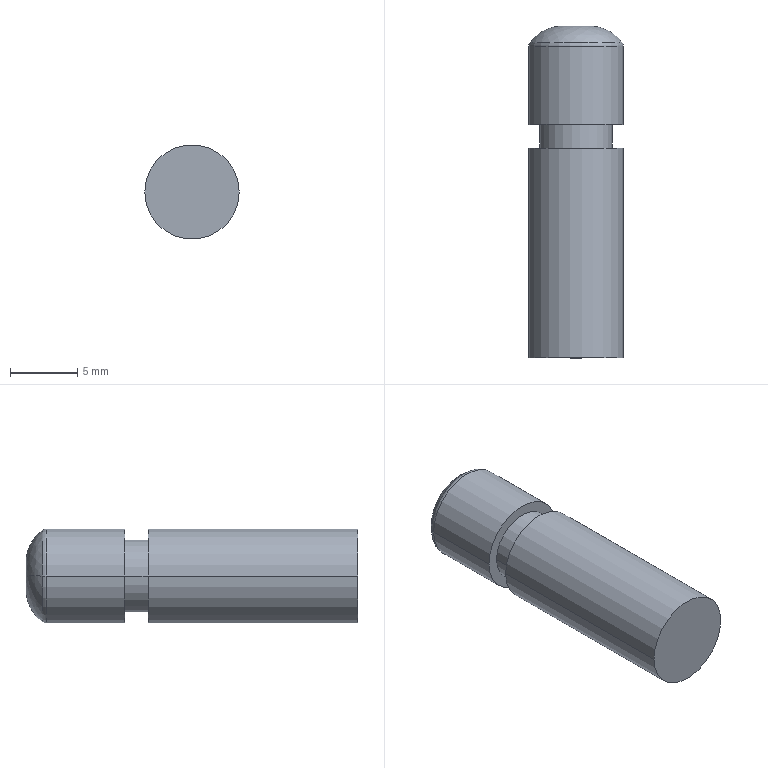Part | STEP file | 2023_07_21_12_39_19_0133 | 1 solid | 14 faces | box 7 x 24.6 x 7 mm | volume 901.225 mm3 | cylinder 6 | plane 4 | spline 2 | torus 2 | commonest cylinder face diameters 7 x4 5.4 x2
STEP:
#1=CARTESIAN_POINT('',(16.5,75.7,12.5));
#2=VERTEX_POINT('',#1);
#3=CARTESIAN_POINT('',(14.5,75.7,12.5));
#4=VERTEX_POINT('',#3);
#5=CARTESIAN_POINT('',(15.5,75.7,12.5));
#6=DIRECTION('',(0.,-1.,0.));
#7=DIRECTION('',(-1.,0.,0.));
#8=AXIS2_PLACEMENT_3D('',#5,#6,#7);
#9=CIRCLE('',#8,1.);
#10=EDGE_CURVE('',#2,#4,#9,.T.);
#11=ORIENTED_EDGE('',*,*,#10,.T.);
#12=CARTESIAN_POINT('',(12.1,74.5,12.5));
#13=VERTEX_POINT('',#12);
#14=CARTESIAN_POINT('',(14.5,75.7,12.5));
#15=CARTESIAN_POINT('',(13.,75.7,12.5));
#16=CARTESIAN_POINT('',(12.1,74.5,12.5));
#17=(BOUNDED_CURVE()B_SPLINE_CURVE(2,(#14,#15,#16),.UNSPECIFIED.,.F.,.F.)B_SPLINE_CURVE_WITH_KNOTS((3,3),(-1.571,-0.6435),.UNSPECIFIED.)CURVE()GEOMETRIC_REPRESENTATION_ITEM()RATIONAL_B_SPLINE_CURVE((1.,0.8944,1.))REPRESENTATION_ITEM(''));
#18=EDGE_CURVE('',#4,#13,#17,.T.);
#19=ORIENTED_EDGE('',*,*,#18,.T.);
#20=CARTESIAN_POINT('',(18.9,74.5,12.5));
#21=VERTEX_POINT('',#20);
#22=CARTESIAN_POINT('',(15.5,74.5,12.5));
#23=DIRECTION('',(0.,-1.,0.));
#24=DIRECTION('',(-1.,0.,0.));
#25=AXIS2_PLACEMENT_3D('',#22,#23,#24);
#26=CIRCLE('',#25,3.4);
#27=EDGE_CURVE('',#21,#13,#26,.T.);
#28=ORIENTED_EDGE('',*,*,#27,.F.);
#29=CARTESIAN_POINT('',(16.5,75.7,12.5));
#30=CARTESIAN_POINT('',(18.,75.7,12.5));
#31=CARTESIAN_POINT('',(18.9,74.5,12.5));
#32=(BOUNDED_CURVE()B_SPLINE_CURVE(2,(#29,#30,#31),.UNSPECIFIED.,.F.,.F.)B_SPLINE_CURVE_WITH_KNOTS((3,3),(-1.571,-0.6435),.UNSPECIFIED.)CURVE()GEOMETRIC_REPRESENTATION_ITEM()RATIONAL_B_SPLINE_CURVE((1.,0.8944,1.))REPRESENTATION_ITEM(''));
#33=EDGE_CURVE('',#2,#21,#32,.T.);
#34=ORIENTED_EDGE('',*,*,#33,.F.);
#35=EDGE_LOOP('',(#11,#19,#28,#34));
#36=FACE_OUTER_BOUND('',#35,.T.);
#37=CARTESIAN_POINT('',(16.5,75.7,12.5));
#38=CARTESIAN_POINT('',(16.5,75.7,13.5));
#39=CARTESIAN_POINT('',(15.5,75.7,13.5));
#40=CARTESIAN_POINT('',(14.5,75.7,13.5));
#41=CARTESIAN_POINT('',(14.5,75.7,12.5));
#42=CARTESIAN_POINT('',(14.5,75.7,11.5));
#43=CARTESIAN_POINT('',(15.5,75.7,11.5));
#44=CARTESIAN_POINT('',(16.5,75.7,11.5));
#45=CARTESIAN_POINT('',(16.5,75.7,12.5));
#46=CARTESIAN_POINT('',(18.,75.7,12.5));
#47=CARTESIAN_POINT('',(18.,75.7,15.));
#48=CARTESIAN_POINT('',(15.5,75.7,15.));
#49=CARTESIAN_POINT('',(13.,75.7,15.));
#50=CARTESIAN_POINT('',(13.,75.7,12.5));
#51=CARTESIAN_POINT('',(13.,75.7,10.));
#52=CARTESIAN_POINT('',(15.5,75.7,10.));
#53=CARTESIAN_POINT('',(18.,75.7,10.));
#54=CARTESIAN_POINT('',(18.,75.7,12.5));
#55=CARTESIAN_POINT('',(18.9,74.5,12.5));
#56=CARTESIAN_POINT('',(18.9,74.5,15.9));
#57=CARTESIAN_POINT('',(15.5,74.5,15.9));
#58=CARTESIAN_POINT('',(12.1,74.5,15.9));
#59=CARTESIAN_POINT('',(12.1,74.5,12.5));
#60=CARTESIAN_POINT('',(12.1,74.5,9.1));
#61=CARTESIAN_POINT('',(15.5,74.5,9.1));
#62=CARTESIAN_POINT('',(18.9,74.5,9.1));
#63=CARTESIAN_POINT('',(18.9,74.5,12.5));
#64=(BOUNDED_SURFACE()B_SPLINE_SURFACE(2,2,((#37,#38,#39,#40,#41,#42,#43,#44,#45),(#46,#47,#48,#49,#50,#51,#52,#53,#54),(#55,#56,#57,#58,#59,#60,#61,#62,#63)),.UNSPECIFIED.,.F.,.T.,.F.)B_SPLINE_SURFACE_WITH_KNOTS((3,3),(3,2,2,2,3),(-1.571,-0.6435),(-3.142,-1.571,0.,1.571,3.142),.UNSPECIFIED.)GEOMETRIC_REPRESENTATION_ITEM()RATIONAL_B_SPLINE_SURFACE(((1.,0.7071,1.,0.7071,1.,0.7071,1.,0.7071,1.),(0.8944,0.6325,0.8944,0.6325,0.8944,0.6325,0.8944,0.6325,0.8944),(1.,0.7071,1.,0.7071,1.,0.7071,1.,0.7071,1.)))REPRESENTATION_ITEM('')SURFACE());
#65=ADVANCED_FACE('',(#36),#64,.F.);
#66=CARTESIAN_POINT('',(19.,51.1,12.5));
#67=VERTEX_POINT('',#66);
#68=CARTESIAN_POINT('',(12.,51.1,12.5));
#69=VERTEX_POINT('',#68);
#70=CARTESIAN_POINT('',(15.5,51.1,12.5));
#71=DIRECTION('',(0.,-1.,0.));
#72=DIRECTION('',(-1.,0.,0.));
#73=AXIS2_PLACEMENT_3D('',#70,#71,#72);
#74=CIRCLE('',#73,3.5);
#75=EDGE_CURVE('',#67,#69,#74,.T.);
#76=ORIENTED_EDGE('',*,*,#75,.F.);
#77=CARTESIAN_POINT('',(19.,66.65,12.5));
#78=VERTEX_POINT('',#77);
#79=CARTESIAN_POINT('',(19.,58.875,12.5));
#80=DIRECTION('',(0.,1.,0.));
#81=VECTOR('',#80,1000.);
#82=LINE('',#79,#81);
#83=EDGE_CURVE('',#67,#78,#82,.T.);
#84=ORIENTED_EDGE('',*,*,#83,.T.);
#85=CARTESIAN_POINT('',(12.,66.65,12.5));
#86=VERTEX_POINT('',#85);
#87=CARTESIAN_POINT('',(15.5,66.65,12.5));
#88=DIRECTION('',(0.,-1.,0.));
#89=DIRECTION('',(-1.,0.,0.));
#90=AXIS2_PLACEMENT_3D('',#87,#88,#89);
#91=CIRCLE('',#90,3.5);
#92=EDGE_CURVE('',#78,#86,#91,.T.);
#93=ORIENTED_EDGE('',*,*,#92,.T.);
#94=CARTESIAN_POINT('',(12.,58.875,12.5));
#95=DIRECTION('',(0.,1.,0.));
#96=VECTOR('',#95,1000.);
#97=LINE('',#94,#96);
#98=EDGE_CURVE('',#69,#86,#97,.T.);
#99=ORIENTED_EDGE('',*,*,#98,.F.);
#100=EDGE_LOOP('',(#76,#84,#93,#99));
#101=FACE_OUTER_BOUND('',#100,.T.);
#102=CARTESIAN_POINT('',(15.5,58.875,12.5));
#103=DIRECTION('',(0.,1.,0.));
#104=DIRECTION('',(-1.,0.,0.));
#105=AXIS2_PLACEMENT_3D('',#102,#103,#104);
#106=CYLINDRICAL_SURFACE('',#105,3.5);
#107=ADVANCED_FACE('',(#101),#106,.T.);
#108=CARTESIAN_POINT('',(18.2,66.65,12.5));
#109=VERTEX_POINT('',#108);
#110=CARTESIAN_POINT('',(12.8,66.65,12.5));
#111=VERTEX_POINT('',#110);
#112=CARTESIAN_POINT('',(15.5,66.65,12.5));
#113=DIRECTION('',(0.,-1.,0.));
#114=DIRECTION('',(-1.,0.,0.));
#115=AXIS2_PLACEMENT_3D('',#112,#113,#114);
#116=CIRCLE('',#115,2.7);
#117=EDGE_CURVE('',#109,#111,#116,.T.);
#118=ORIENTED_EDGE('',*,*,#117,.F.);
#119=CARTESIAN_POINT('',(18.2,68.4,12.5));
#120=VERTEX_POINT('',#119);
#121=CARTESIAN_POINT('',(18.2,67.525,12.5));
#122=DIRECTION('',(0.,1.,0.));
#123=VECTOR('',#122,1000.);
#124=LINE('',#121,#123);
#125=EDGE_CURVE('',#109,#120,#124,.T.);
#126=ORIENTED_EDGE('',*,*,#125,.T.);
#127=CARTESIAN_POINT('',(12.8,68.4,12.5));
#128=VERTEX_POINT('',#127);
#129=CARTESIAN_POINT('',(15.5,68.4,12.5));
#130=DIRECTION('',(0.,-1.,0.));
#131=DIRECTION('',(-1.,0.,0.));
#132=AXIS2_PLACEMENT_3D('',#129,#130,#131);
#133=CIRCLE('',#132,2.7);
#134=EDGE_CURVE('',#120,#128,#133,.T.);
#135=ORIENTED_EDGE('',*,*,#134,.T.);
#136=CARTESIAN_POINT('',(12.8,67.525,12.5));
#137=DIRECTION('',(0.,1.,0.));
#138=VECTOR('',#137,1000.);
#139=LINE('',#136,#138);
#140=EDGE_CURVE('',#111,#128,#139,.T.);
#141=ORIENTED_EDGE('',*,*,#140,.F.);
#142=EDGE_LOOP('',(#118,#126,#135,#141));
#143=FACE_OUTER_BOUND('',#142,.T.);
#144=CARTESIAN_POINT('',(15.5,67.525,12.5));
#145=DIRECTION('',(0.,1.,0.));
#146=DIRECTION('',(-1.,0.,0.));
#147=AXIS2_PLACEMENT_3D('',#144,#145,#146);
#148=CYLINDRICAL_SURFACE('',#147,2.7);
#149=ADVANCED_FACE('',(#143),#148,.T.);
#150=CARTESIAN_POINT('',(19.,68.4,12.5));
#151=VERTEX_POINT('',#150);
#152=CARTESIAN_POINT('',(12.,68.4,12.5));
#153=VERTEX_POINT('',#152);
#154=CARTESIAN_POINT('',(15.5,68.4,12.5));
#155=DIRECTION('',(0.,-1.,0.));
#156=DIRECTION('',(-1.,0.,0.));
#157=AXIS2_PLACEMENT_3D('',#154,#155,#156);
#158=CIRCLE('',#157,3.5);
#159=EDGE_CURVE('',#151,#153,#158,.T.);
#160=ORIENTED_EDGE('',*,*,#159,.F.);
#161=CARTESIAN_POINT('',(19.,74.2,12.5));
#162=VERTEX_POINT('',#161);
#163=CARTESIAN_POINT('',(19.,71.3,12.5));
#164=DIRECTION('',(0.,1.,0.));
#165=VECTOR('',#164,1000.);
#166=LINE('',#163,#165);
#167=EDGE_CURVE('',#151,#162,#166,.T.);
#168=ORIENTED_EDGE('',*,*,#167,.T.);
#169=CARTESIAN_POINT('',(12.,74.2,12.5));
#170=VERTEX_POINT('',#169);
#171=CARTESIAN_POINT('',(15.5,74.2,12.5));
#172=DIRECTION('',(0.,-1.,0.));
#173=DIRECTION('',(-1.,0.,0.));
#174=AXIS2_PLACEMENT_3D('',#171,#172,#173);
#175=CIRCLE('',#174,3.5);
#176=EDGE_CURVE('',#162,#170,#175,.T.);
#177=ORIENTED_EDGE('',*,*,#176,.T.);
#178=CARTESIAN_POINT('',(12.,71.3,12.5));
#179=DIRECTION('',(0.,1.,0.));
#180=VECTOR('',#179,1000.);
#181=LINE('',#178,#180);
#182=EDGE_CURVE('',#153,#170,#181,.T.);
#183=ORIENTED_EDGE('',*,*,#182,.F.);
#184=EDGE_LOOP('',(#160,#168,#177,#183));
#185=FACE_OUTER_BOUND('',#184,.T.);
#186=CARTESIAN_POINT('',(15.5,71.3,12.5));
#187=DIRECTION('',(0.,1.,0.));
#188=DIRECTION('',(-1.,0.,0.));
#189=AXIS2_PLACEMENT_3D('',#186,#187,#188);
#190=CYLINDRICAL_SURFACE('',#189,3.5);
#191=ADVANCED_FACE('',(#185),#190,.T.);
#192=CARTESIAN_POINT('',(15.5,74.5,12.5));
#193=DIRECTION('',(0.,-1.,0.));
#194=DIRECTION('',(-1.,0.,0.));
#195=AXIS2_PLACEMENT_3D('',#192,#193,#194);
#196=CIRCLE('',#195,3.4);
#197=EDGE_CURVE('',#13,#21,#196,.T.);
#198=ORIENTED_EDGE('',*,*,#197,.T.);
#199=CARTESIAN_POINT('',(18.5,74.2,12.5));
#200=DIRECTION('',(0.,0.,-1.));
#201=DIRECTION('',(-1.,0.,0.));
#202=AXIS2_PLACEMENT_3D('',#199,#200,#201);
#203=CIRCLE('',#202,0.5);
#204=EDGE_CURVE('',#21,#162,#203,.T.);
#205=ORIENTED_EDGE('',*,*,#204,.T.);
#206=CARTESIAN_POINT('',(15.5,74.2,12.5));
#207=DIRECTION('',(0.,-1.,0.));
#208=DIRECTION('',(-1.,0.,0.));
#209=AXIS2_PLACEMENT_3D('',#206,#207,#208);
#210=CIRCLE('',#209,3.5);
#211=EDGE_CURVE('',#170,#162,#210,.T.);
#212=ORIENTED_EDGE('',*,*,#211,.F.);
#213=CARTESIAN_POINT('',(12.5,74.2,12.5));
#214=DIRECTION('',(0.,0.,1.));
#215=DIRECTION('',(1.,0.,0.));
#216=AXIS2_PLACEMENT_3D('',#213,#214,#215);
#217=CIRCLE('',#216,0.5);
#218=EDGE_CURVE('',#13,#170,#217,.T.);
#219=ORIENTED_EDGE('',*,*,#218,.F.);
#220=EDGE_LOOP('',(#198,#205,#212,#219));
#221=FACE_OUTER_BOUND('',#220,.T.);
#222=CARTESIAN_POINT('',(15.5,74.2,12.5));
#223=DIRECTION('',(0.,-1.,0.));
#224=DIRECTION('',(-1.,0.,0.));
#225=AXIS2_PLACEMENT_3D('',#222,#223,#224);
#226=TOROIDAL_SURFACE('',#225,3.,0.5);
#227=ADVANCED_FACE('',(#221),#226,.T.);
#228=ORIENTED_EDGE('',*,*,#10,.F.);
#229=CARTESIAN_POINT('',(15.5,75.7,12.5));
#230=DIRECTION('',(0.,-1.,0.));
#231=DIRECTION('',(-1.,0.,0.));
#232=AXIS2_PLACEMENT_3D('',#229,#230,#231);
#233=CIRCLE('',#232,1.);
#234=EDGE_CURVE('',#4,#2,#233,.T.);
#235=ORIENTED_EDGE('',*,*,#234,.F.);
#236=EDGE_LOOP('',(#228,#235));
#237=FACE_OUTER_BOUND('',#236,.T.);
#238=CARTESIAN_POINT('',(15.,75.7,12.5));
#239=DIRECTION('',(0.,1.,0.));
#240=DIRECTION('',(1.,0.,0.));
#241=AXIS2_PLACEMENT_3D('',#238,#239,#240);
#242=PLANE('',#241);
#243=ADVANCED_FACE('',(#237),#242,.T.);
#244=CARTESIAN_POINT('',(15.5,51.1,12.5));
#245=DIRECTION('',(0.,-1.,0.));
#246=DIRECTION('',(-1.,0.,0.));
#247=AXIS2_PLACEMENT_3D('',#244,#245,#246);
#248=CIRCLE('',#247,3.5);
#249=EDGE_CURVE('',#69,#67,#248,.T.);
#250=ORIENTED_EDGE('',*,*,#249,.T.);
#251=ORIENTED_EDGE('',*,*,#75,.T.);
#252=EDGE_LOOP('',(#250,#251));
#253=FACE_OUTER_BOUND('',#252,.T.);
#254=CARTESIAN_POINT('',(13.75,51.1,12.5));
#255=DIRECTION('',(0.,-1.,0.));
#256=DIRECTION('',(0.,0.,-1.));
#257=AXIS2_PLACEMENT_3D('',#254,#255,#256);
#258=PLANE('',#257);
#259=ADVANCED_FACE('',(#253),#258,.T.);
#260=CARTESIAN_POINT('',(15.5,66.65,12.5));
#261=DIRECTION('',(0.,-1.,0.));
#262=DIRECTION('',(-1.,0.,0.));
#263=AXIS2_PLACEMENT_3D('',#260,#261,#262);
#264=CIRCLE('',#263,2.7);
#265=EDGE_CURVE('',#111,#109,#264,.T.);
#266=ORIENTED_EDGE('',*,*,#265,.T.);
#267=ORIENTED_EDGE('',*,*,#117,.T.);
#268=EDGE_LOOP('',(#266,#267));
#269=FACE_BOUND('',#268,.T.);
#270=CARTESIAN_POINT('',(15.5,66.65,12.5));
#271=DIRECTION('',(0.,-1.,0.));
#272=DIRECTION('',(-1.,0.,0.));
#273=AXIS2_PLACEMENT_3D('',#270,#271,#272);
#274=CIRCLE('',#273,3.5);
#275=EDGE_CURVE('',#86,#78,#274,.T.);
#276=ORIENTED_EDGE('',*,*,#275,.F.);
#277=ORIENTED_EDGE('',*,*,#92,.F.);
#278=EDGE_LOOP('',(#276,#277));
#279=FACE_OUTER_BOUND('',#278,.T.);
#280=CARTESIAN_POINT('',(12.4,66.65,12.5));
#281=DIRECTION('',(0.,1.,0.));
#282=DIRECTION('',(1.,0.,0.));
#283=AXIS2_PLACEMENT_3D('',#280,#281,#282);
#284=PLANE('',#283);
#285=ADVANCED_FACE('',(#269,#279),#284,.T.);
#286=CARTESIAN_POINT('',(15.5,68.4,12.5));
#287=DIRECTION('',(0.,-1.,0.));
#288=DIRECTION('',(-1.,0.,0.));
#289=AXIS2_PLACEMENT_3D('',#286,#287,#288);
#290=CIRCLE('',#289,2.7);
#291=EDGE_CURVE('',#128,#120,#290,.T.);
#292=ORIENTED_EDGE('',*,*,#291,.F.);
#293=ORIENTED_EDGE('',*,*,#134,.F.);
#294=EDGE_LOOP('',(#292,#293));
#295=FACE_BOUND('',#294,.T.);
#296=CARTESIAN_POINT('',(15.5,68.4,12.5));
#297=DIRECTION('',(0.,-1.,0.));
#298=DIRECTION('',(-1.,0.,0.));
#299=AXIS2_PLACEMENT_3D('',#296,#297,#298);
#300=CIRCLE('',#299,3.5);
#301=EDGE_CURVE('',#153,#151,#300,.T.);
#302=ORIENTED_EDGE('',*,*,#301,.T.);
#303=ORIENTED_EDGE('',*,*,#159,.T.);
#304=EDGE_LOOP('',(#302,#303));
#305=FACE_OUTER_BOUND('',#304,.T.);
#306=CARTESIAN_POINT('',(12.4,68.4,12.5));
#307=DIRECTION('',(0.,-1.,0.));
#308=DIRECTION('',(0.,0.,-1.));
#309=AXIS2_PLACEMENT_3D('',#306,#307,#308);
#310=PLANE('',#309);
#311=ADVANCED_FACE('',(#295,#305),#310,.T.);
#312=ORIENTED_EDGE('',*,*,#18,.F.);
#313=ORIENTED_EDGE('',*,*,#234,.T.);
#314=ORIENTED_EDGE('',*,*,#33,.T.);
#315=ORIENTED_EDGE('',*,*,#197,.F.);
#316=EDGE_LOOP('',(#312,#313,#314,#315));
#317=FACE_OUTER_BOUND('',#316,.T.);
#318=CARTESIAN_POINT('',(16.5,75.7,12.5));
#319=CARTESIAN_POINT('',(16.5,75.7,13.5));
#320=CARTESIAN_POINT('',(15.5,75.7,13.5));
#321=CARTESIAN_POINT('',(14.5,75.7,13.5));
#322=CARTESIAN_POINT('',(14.5,75.7,12.5));
#323=CARTESIAN_POINT('',(14.5,75.7,11.5));
#324=CARTESIAN_POINT('',(15.5,75.7,11.5));
#325=CARTESIAN_POINT('',(16.5,75.7,11.5));
#326=CARTESIAN_POINT('',(16.5,75.7,12.5));
#327=CARTESIAN_POINT('',(18.,75.7,12.5));
#328=CARTESIAN_POINT('',(18.,75.7,15.));
#329=CARTESIAN_POINT('',(15.5,75.7,15.));
#330=CARTESIAN_POINT('',(13.,75.7,15.));
#331=CARTESIAN_POINT('',(13.,75.7,12.5));
#332=CARTESIAN_POINT('',(13.,75.7,10.));
#333=CARTESIAN_POINT('',(15.5,75.7,10.));
#334=CARTESIAN_POINT('',(18.,75.7,10.));
#335=CARTESIAN_POINT('',(18.,75.7,12.5));
#336=CARTESIAN_POINT('',(18.9,74.5,12.5));
#337=CARTESIAN_POINT('',(18.9,74.5,15.9));
#338=CARTESIAN_POINT('',(15.5,74.5,15.9));
#339=CARTESIAN_POINT('',(12.1,74.5,15.9));
#340=CARTESIAN_POINT('',(12.1,74.5,12.5));
#341=CARTESIAN_POINT('',(12.1,74.5,9.1));
#342=CARTESIAN_POINT('',(15.5,74.5,9.1));
#343=CARTESIAN_POINT('',(18.9,74.5,9.1));
#344=CARTESIAN_POINT('',(18.9,74.5,12.5));
#345=(BOUNDED_SURFACE()B_SPLINE_SURFACE(2,2,((#318,#319,#320,#321,#322,#323,#324,#325,#326),(#327,#328,#329,#330,#331,#332,#333,#334,#335),(#336,#337,#338,#339,#340,#341,#342,#343,#344)),.UNSPECIFIED.,.F.,.T.,.F.)B_SPLINE_SURFACE_WITH_KNOTS((3,3),(3,2,2,2,3),(-1.571,-0.6435),(-3.142,-1.571,0.,1.571,3.142),.UNSPECIFIED.)GEOMETRIC_REPRESENTATION_ITEM()RATIONAL_B_SPLINE_SURFACE(((1.,0.7071,1.,0.7071,1.,0.7071,1.,0.7071,1.),(0.8944,0.6325,0.8944,0.6325,0.8944,0.6325,0.8944,0.6325,0.8944),(1.,0.7071,1.,0.7071,1.,0.7071,1.,0.7071,1.)))REPRESENTATION_ITEM('')SURFACE());
#346=ADVANCED_FACE('',(#317),#345,.F.);
#347=ORIENTED_EDGE('',*,*,#204,.F.);
#348=ORIENTED_EDGE('',*,*,#27,.T.);
#349=ORIENTED_EDGE('',*,*,#218,.T.);
#350=ORIENTED_EDGE('',*,*,#176,.F.);
#351=EDGE_LOOP('',(#347,#348,#349,#350));
#352=FACE_OUTER_BOUND('',#351,.T.);
#353=CARTESIAN_POINT('',(15.5,74.2,12.5));
#354=DIRECTION('',(0.,-1.,0.));
#355=DIRECTION('',(-1.,0.,0.));
#356=AXIS2_PLACEMENT_3D('',#353,#354,#355);
#357=TOROIDAL_SURFACE('',#356,3.,0.5);
#358=ADVANCED_FACE('',(#352),#357,.T.);
#359=ORIENTED_EDGE('',*,*,#167,.F.);
#360=ORIENTED_EDGE('',*,*,#301,.F.);
#361=ORIENTED_EDGE('',*,*,#182,.T.);
#362=ORIENTED_EDGE('',*,*,#211,.T.);
#363=EDGE_LOOP('',(#359,#360,#361,#362));
#364=FACE_OUTER_BOUND('',#363,.T.);
#365=CARTESIAN_POINT('',(15.5,71.3,12.5));
#366=DIRECTION('',(0.,1.,0.));
#367=DIRECTION('',(-1.,0.,0.));
#368=AXIS2_PLACEMENT_3D('',#365,#366,#367);
#369=CYLINDRICAL_SURFACE('',#368,3.5);
#370=ADVANCED_FACE('',(#364),#369,.T.);
#371=ORIENTED_EDGE('',*,*,#125,.F.);
#372=ORIENTED_EDGE('',*,*,#265,.F.);
#373=ORIENTED_EDGE('',*,*,#140,.T.);
#374=ORIENTED_EDGE('',*,*,#291,.T.);
#375=EDGE_LOOP('',(#371,#372,#373,#374));
#376=FACE_OUTER_BOUND('',#375,.T.);
#377=CARTESIAN_POINT('',(15.5,67.525,12.5));
#378=DIRECTION('',(0.,1.,0.));
#379=DIRECTION('',(-1.,0.,0.));
#380=AXIS2_PLACEMENT_3D('',#377,#378,#379);
#381=CYLINDRICAL_SURFACE('',#380,2.7);
#382=ADVANCED_FACE('',(#376),#381,.T.);
#383=ORIENTED_EDGE('',*,*,#83,.F.);
#384=ORIENTED_EDGE('',*,*,#249,.F.);
#385=ORIENTED_EDGE('',*,*,#98,.T.);
#386=ORIENTED_EDGE('',*,*,#275,.T.);
#387=EDGE_LOOP('',(#383,#384,#385,#386));
#388=FACE_OUTER_BOUND('',#387,.T.);
#389=CARTESIAN_POINT('',(15.5,58.875,12.5));
#390=DIRECTION('',(0.,1.,0.));
#391=DIRECTION('',(-1.,0.,0.));
#392=AXIS2_PLACEMENT_3D('',#389,#390,#391);
#393=CYLINDRICAL_SURFACE('',#392,3.5);
#394=ADVANCED_FACE('',(#388),#393,.T.);
#395=CLOSED_SHELL('',(#65,#107,#149,#191,#227,#243,#259,#285,#311,#346,#358,#370,#382,#394));
#396=MANIFOLD_SOLID_BREP('',#395);
#397=CARTESIAN_POINT('',(0.,0.,0.));
#398=DIRECTION('',(0.,0.,1.));
#399=DIRECTION('',(1.,0.,0.));
#400=AXIS2_PLACEMENT_3D('',#397,#398,#399);
#401=(LENGTH_UNIT()NAMED_UNIT(*)SI_UNIT(.MILLI.,.METRE.));
#402=UNCERTAINTY_MEASURE_WITH_UNIT(LENGTH_MEASURE(0.00001),#401,'','');
#403=(NAMED_UNIT(*)PLANE_ANGLE_UNIT()SI_UNIT($,.RADIAN.));
#404=(NAMED_UNIT(*)SI_UNIT($,.STERADIAN.)SOLID_ANGLE_UNIT());
#405=(GEOMETRIC_REPRESENTATION_CONTEXT(3)GLOBAL_UNCERTAINTY_ASSIGNED_CONTEXT((#402))GLOBAL_UNIT_ASSIGNED_CONTEXT((#401,#403,#404))REPRESENTATION_CONTEXT('',''));
#406=ADVANCED_BREP_SHAPE_REPRESENTATION('',(#396,#400),#405);